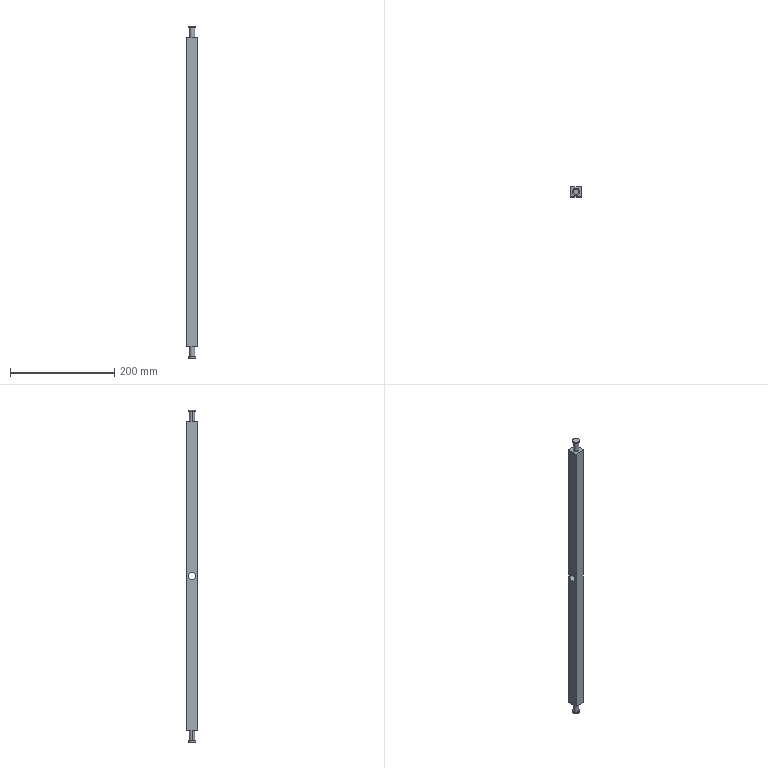Part | SolidWorks | 1 solid | 20 faces | box 20 x 20 x 638 mm | volume 238279 mm3 | cylinder 10 | plane 10 | commonest cylinder face diameters 14 x6 10 x4
STEP:
#1=CARTESIAN_POINT('',(-10.,-7.,0.));
#2=VERTEX_POINT('',#1);
#3=CARTESIAN_POINT('',(-10.,7.,0.));
#4=VERTEX_POINT('',#3);
#5=CARTESIAN_POINT('',(-10.,0.,0.));
#6=DIRECTION('',(1.,0.,0.));
#7=DIRECTION('',(0.,1.,0.));
#8=AXIS2_PLACEMENT_3D('',#5,#6,#7);
#9=CIRCLE('',#8,7.);
#10=EDGE_CURVE('',#2,#4,#9,.T.);
#11=ORIENTED_EDGE('',*,*,#10,.F.);
#12=CARTESIAN_POINT('',(10.,-7.,0.));
#13=VERTEX_POINT('',#12);
#14=CARTESIAN_POINT('',(-46.,-7.,0.));
#15=DIRECTION('',(1.,0.,0.));
#16=VECTOR('',#15,1000.);
#17=LINE('',#14,#16);
#18=EDGE_CURVE('',#2,#13,#17,.T.);
#19=ORIENTED_EDGE('',*,*,#18,.T.);
#20=CARTESIAN_POINT('',(10.,7.,0.));
#21=VERTEX_POINT('',#20);
#22=CARTESIAN_POINT('',(10.,0.,0.));
#23=DIRECTION('',(1.,0.,0.));
#24=DIRECTION('',(0.,1.,0.));
#25=AXIS2_PLACEMENT_3D('',#22,#23,#24);
#26=CIRCLE('',#25,7.);
#27=EDGE_CURVE('',#13,#21,#26,.T.);
#28=ORIENTED_EDGE('',*,*,#27,.T.);
#29=CARTESIAN_POINT('',(-46.,7.,0.));
#30=DIRECTION('',(1.,0.,0.));
#31=VECTOR('',#30,1000.);
#32=LINE('',#29,#31);
#33=EDGE_CURVE('',#4,#21,#32,.T.);
#34=ORIENTED_EDGE('',*,*,#33,.F.);
#35=EDGE_LOOP('',(#11,#19,#28,#34));
#36=FACE_OUTER_BOUND('',#35,.T.);
#37=CARTESIAN_POINT('',(-46.,0.,0.));
#38=DIRECTION('',(1.,0.,0.));
#39=DIRECTION('',(0.,1.,0.));
#40=AXIS2_PLACEMENT_3D('',#37,#38,#39);
#41=CYLINDRICAL_SURFACE('',#40,7.);
#42=ADVANCED_FACE('',(#36),#41,.F.);
#43=CARTESIAN_POINT('',(7.,0.,-319.));
#44=VERTEX_POINT('',#43);
#45=CARTESIAN_POINT('',(-7.,0.,-319.));
#46=VERTEX_POINT('',#45);
#47=CARTESIAN_POINT('',(0.,0.,-319.));
#48=DIRECTION('',(0.,0.,1.));
#49=DIRECTION('',(1.,0.,0.));
#50=AXIS2_PLACEMENT_3D('',#47,#48,#49);
#51=CIRCLE('',#50,7.);
#52=EDGE_CURVE('',#44,#46,#51,.T.);
#53=ORIENTED_EDGE('',*,*,#52,.T.);
#54=CARTESIAN_POINT('',(-7.,0.,-317.));
#55=VERTEX_POINT('',#54);
#56=CARTESIAN_POINT('',(-7.,0.,-319.));
#57=DIRECTION('',(0.,0.,1.));
#58=VECTOR('',#57,1000.);
#59=LINE('',#56,#58);
#60=EDGE_CURVE('',#46,#55,#59,.T.);
#61=ORIENTED_EDGE('',*,*,#60,.T.);
#62=CARTESIAN_POINT('',(7.,0.,-317.));
#63=VERTEX_POINT('',#62);
#64=CARTESIAN_POINT('',(0.,0.,-317.));
#65=DIRECTION('',(0.,0.,1.));
#66=DIRECTION('',(1.,0.,0.));
#67=AXIS2_PLACEMENT_3D('',#64,#65,#66);
#68=CIRCLE('',#67,7.);
#69=EDGE_CURVE('',#63,#55,#68,.T.);
#70=ORIENTED_EDGE('',*,*,#69,.F.);
#71=CARTESIAN_POINT('',(7.,0.,-319.));
#72=DIRECTION('',(0.,0.,1.));
#73=VECTOR('',#72,1000.);
#74=LINE('',#71,#73);
#75=EDGE_CURVE('',#44,#63,#74,.T.);
#76=ORIENTED_EDGE('',*,*,#75,.F.);
#77=EDGE_LOOP('',(#53,#61,#70,#76));
#78=FACE_OUTER_BOUND('',#77,.T.);
#79=CARTESIAN_POINT('',(0.,0.,-319.));
#80=DIRECTION('',(0.,0.,1.));
#81=DIRECTION('',(1.,0.,0.));
#82=AXIS2_PLACEMENT_3D('',#79,#80,#81);
#83=CYLINDRICAL_SURFACE('',#82,7.);
#84=ADVANCED_FACE('',(#78),#83,.T.);
#85=CARTESIAN_POINT('',(5.,0.,-317.));
#86=VERTEX_POINT('',#85);
#87=CARTESIAN_POINT('',(-5.,0.,-317.));
#88=VERTEX_POINT('',#87);
#89=CARTESIAN_POINT('',(0.,0.,-317.));
#90=DIRECTION('',(0.,0.,1.));
#91=DIRECTION('',(1.,0.,0.));
#92=AXIS2_PLACEMENT_3D('',#89,#90,#91);
#93=CIRCLE('',#92,5.);
#94=EDGE_CURVE('',#86,#88,#93,.T.);
#95=ORIENTED_EDGE('',*,*,#94,.T.);
#96=CARTESIAN_POINT('',(-5.,0.,-297.));
#97=VERTEX_POINT('',#96);
#98=CARTESIAN_POINT('',(-5.,0.,-317.));
#99=DIRECTION('',(0.,0.,1.));
#100=VECTOR('',#99,1000.);
#101=LINE('',#98,#100);
#102=EDGE_CURVE('',#88,#97,#101,.T.);
#103=ORIENTED_EDGE('',*,*,#102,.T.);
#104=CARTESIAN_POINT('',(5.,0.,-297.));
#105=VERTEX_POINT('',#104);
#106=CARTESIAN_POINT('',(0.,0.,-297.));
#107=DIRECTION('',(0.,0.,1.));
#108=DIRECTION('',(1.,0.,0.));
#109=AXIS2_PLACEMENT_3D('',#106,#107,#108);
#110=CIRCLE('',#109,5.);
#111=EDGE_CURVE('',#105,#97,#110,.T.);
#112=ORIENTED_EDGE('',*,*,#111,.F.);
#113=CARTESIAN_POINT('',(5.,0.,-317.));
#114=DIRECTION('',(0.,0.,1.));
#115=VECTOR('',#114,1000.);
#116=LINE('',#113,#115);
#117=EDGE_CURVE('',#86,#105,#116,.T.);
#118=ORIENTED_EDGE('',*,*,#117,.F.);
#119=EDGE_LOOP('',(#95,#103,#112,#118));
#120=FACE_OUTER_BOUND('',#119,.T.);
#121=CARTESIAN_POINT('',(0.,0.,-317.));
#122=DIRECTION('',(0.,0.,1.));
#123=DIRECTION('',(1.,0.,0.));
#124=AXIS2_PLACEMENT_3D('',#121,#122,#123);
#125=CYLINDRICAL_SURFACE('',#124,5.);
#126=ADVANCED_FACE('',(#120),#125,.T.);
#127=CARTESIAN_POINT('',(7.,0.,319.));
#128=VERTEX_POINT('',#127);
#129=CARTESIAN_POINT('',(-7.,0.,319.));
#130=VERTEX_POINT('',#129);
#131=CARTESIAN_POINT('',(0.,0.,319.));
#132=DIRECTION('',(0.,0.,1.));
#133=DIRECTION('',(1.,0.,0.));
#134=AXIS2_PLACEMENT_3D('',#131,#132,#133);
#135=CIRCLE('',#134,7.);
#136=EDGE_CURVE('',#128,#130,#135,.T.);
#137=ORIENTED_EDGE('',*,*,#136,.F.);
#138=CARTESIAN_POINT('',(7.,0.,317.));
#139=VERTEX_POINT('',#138);
#140=CARTESIAN_POINT('',(7.,0.,319.));
#141=DIRECTION('',(0.,0.,-1.));
#142=VECTOR('',#141,1000.);
#143=LINE('',#140,#142);
#144=EDGE_CURVE('',#128,#139,#143,.T.);
#145=ORIENTED_EDGE('',*,*,#144,.T.);
#146=CARTESIAN_POINT('',(-7.,0.,317.));
#147=VERTEX_POINT('',#146);
#148=CARTESIAN_POINT('',(0.,0.,317.));
#149=DIRECTION('',(0.,0.,1.));
#150=DIRECTION('',(1.,0.,0.));
#151=AXIS2_PLACEMENT_3D('',#148,#149,#150);
#152=CIRCLE('',#151,7.);
#153=EDGE_CURVE('',#139,#147,#152,.T.);
#154=ORIENTED_EDGE('',*,*,#153,.T.);
#155=CARTESIAN_POINT('',(-7.,0.,319.));
#156=DIRECTION('',(0.,0.,-1.));
#157=VECTOR('',#156,1000.);
#158=LINE('',#155,#157);
#159=EDGE_CURVE('',#130,#147,#158,.T.);
#160=ORIENTED_EDGE('',*,*,#159,.F.);
#161=EDGE_LOOP('',(#137,#145,#154,#160));
#162=FACE_OUTER_BOUND('',#161,.T.);
#163=CARTESIAN_POINT('',(0.,0.,319.));
#164=DIRECTION('',(0.,0.,-1.));
#165=DIRECTION('',(-1.,0.,0.));
#166=AXIS2_PLACEMENT_3D('',#163,#164,#165);
#167=CYLINDRICAL_SURFACE('',#166,7.);
#168=ADVANCED_FACE('',(#162),#167,.T.);
#169=CARTESIAN_POINT('',(5.,0.,317.));
#170=VERTEX_POINT('',#169);
#171=CARTESIAN_POINT('',(-5.,0.,317.));
#172=VERTEX_POINT('',#171);
#173=CARTESIAN_POINT('',(0.,0.,317.));
#174=DIRECTION('',(0.,0.,1.));
#175=DIRECTION('',(1.,0.,0.));
#176=AXIS2_PLACEMENT_3D('',#173,#174,#175);
#177=CIRCLE('',#176,5.);
#178=EDGE_CURVE('',#170,#172,#177,.T.);
#179=ORIENTED_EDGE('',*,*,#178,.F.);
#180=CARTESIAN_POINT('',(5.,0.,297.));
#181=VERTEX_POINT('',#180);
#182=CARTESIAN_POINT('',(5.,0.,317.));
#183=DIRECTION('',(0.,0.,-1.));
#184=VECTOR('',#183,1000.);
#185=LINE('',#182,#184);
#186=EDGE_CURVE('',#170,#181,#185,.T.);
#187=ORIENTED_EDGE('',*,*,#186,.T.);
#188=CARTESIAN_POINT('',(-5.,0.,297.));
#189=VERTEX_POINT('',#188);
#190=CARTESIAN_POINT('',(0.,0.,297.));
#191=DIRECTION('',(0.,0.,1.));
#192=DIRECTION('',(1.,0.,0.));
#193=AXIS2_PLACEMENT_3D('',#190,#191,#192);
#194=CIRCLE('',#193,5.);
#195=EDGE_CURVE('',#181,#189,#194,.T.);
#196=ORIENTED_EDGE('',*,*,#195,.T.);
#197=CARTESIAN_POINT('',(-5.,0.,317.));
#198=DIRECTION('',(0.,0.,-1.));
#199=VECTOR('',#198,1000.);
#200=LINE('',#197,#199);
#201=EDGE_CURVE('',#172,#189,#200,.T.);
#202=ORIENTED_EDGE('',*,*,#201,.F.);
#203=EDGE_LOOP('',(#179,#187,#196,#202));
#204=FACE_OUTER_BOUND('',#203,.T.);
#205=CARTESIAN_POINT('',(0.,0.,317.));
#206=DIRECTION('',(0.,0.,-1.));
#207=DIRECTION('',(-1.,0.,0.));
#208=AXIS2_PLACEMENT_3D('',#205,#206,#207);
#209=CYLINDRICAL_SURFACE('',#208,5.);
#210=ADVANCED_FACE('',(#204),#209,.T.);
#211=CARTESIAN_POINT('',(10.,0.,0.));
#212=DIRECTION('',(1.,0.,0.));
#213=DIRECTION('',(0.,1.,0.));
#214=AXIS2_PLACEMENT_3D('',#211,#212,#213);
#215=CIRCLE('',#214,7.);
#216=EDGE_CURVE('',#21,#13,#215,.T.);
#217=ORIENTED_EDGE('',*,*,#216,.F.);
#218=ORIENTED_EDGE('',*,*,#27,.F.);
#219=EDGE_LOOP('',(#217,#218));
#220=FACE_BOUND('',#219,.T.);
#221=CARTESIAN_POINT('',(10.,-10.,-297.));
#222=VERTEX_POINT('',#221);
#223=CARTESIAN_POINT('',(10.,10.,-297.));
#224=VERTEX_POINT('',#223);
#225=CARTESIAN_POINT('',(10.,10.,-297.));
#226=DIRECTION('',(0.,1.,0.));
#227=VECTOR('',#226,1000.);
#228=LINE('',#225,#227);
#229=EDGE_CURVE('',#222,#224,#228,.T.);
#230=ORIENTED_EDGE('',*,*,#229,.T.);
#231=CARTESIAN_POINT('',(10.,10.,297.));
#232=VERTEX_POINT('',#231);
#233=CARTESIAN_POINT('',(10.,10.,297.));
#234=DIRECTION('',(0.,0.,-1.));
#235=VECTOR('',#234,1000.);
#236=LINE('',#233,#235);
#237=EDGE_CURVE('',#232,#224,#236,.T.);
#238=ORIENTED_EDGE('',*,*,#237,.F.);
#239=CARTESIAN_POINT('',(10.,-10.,297.));
#240=VERTEX_POINT('',#239);
#241=CARTESIAN_POINT('',(10.,10.,297.));
#242=DIRECTION('',(0.,1.,0.));
#243=VECTOR('',#242,1000.);
#244=LINE('',#241,#243);
#245=EDGE_CURVE('',#240,#232,#244,.T.);
#246=ORIENTED_EDGE('',*,*,#245,.F.);
#247=CARTESIAN_POINT('',(10.,-10.,297.));
#248=DIRECTION('',(0.,0.,-1.));
#249=VECTOR('',#248,1000.);
#250=LINE('',#247,#249);
#251=EDGE_CURVE('',#240,#222,#250,.T.);
#252=ORIENTED_EDGE('',*,*,#251,.T.);
#253=EDGE_LOOP('',(#230,#238,#246,#252));
#254=FACE_OUTER_BOUND('',#253,.T.);
#255=CARTESIAN_POINT('',(10.,10.,297.));
#256=DIRECTION('',(-1.,0.,0.));
#257=DIRECTION('',(0.,-1.,0.));
#258=AXIS2_PLACEMENT_3D('',#255,#256,#257);
#259=PLANE('',#258);
#260=ADVANCED_FACE('',(#220,#254),#259,.F.);
#261=CARTESIAN_POINT('',(-10.,10.,-297.));
#262=VERTEX_POINT('',#261);
#263=CARTESIAN_POINT('',(-10.,10.,-297.));
#264=DIRECTION('',(-1.,0.,0.));
#265=VECTOR('',#264,1000.);
#266=LINE('',#263,#265);
#267=EDGE_CURVE('',#224,#262,#266,.T.);
#268=ORIENTED_EDGE('',*,*,#267,.T.);
#269=CARTESIAN_POINT('',(-10.,10.,297.));
#270=VERTEX_POINT('',#269);
#271=CARTESIAN_POINT('',(-10.,10.,297.));
#272=DIRECTION('',(0.,0.,-1.));
#273=VECTOR('',#272,1000.);
#274=LINE('',#271,#273);
#275=EDGE_CURVE('',#270,#262,#274,.T.);
#276=ORIENTED_EDGE('',*,*,#275,.F.);
#277=CARTESIAN_POINT('',(-10.,10.,297.));
#278=DIRECTION('',(-1.,0.,0.));
#279=VECTOR('',#278,1000.);
#280=LINE('',#277,#279);
#281=EDGE_CURVE('',#232,#270,#280,.T.);
#282=ORIENTED_EDGE('',*,*,#281,.F.);
#283=ORIENTED_EDGE('',*,*,#237,.T.);
#284=EDGE_LOOP('',(#268,#276,#282,#283));
#285=FACE_OUTER_BOUND('',#284,.T.);
#286=CARTESIAN_POINT('',(-10.,10.,297.));
#287=DIRECTION('',(0.,-1.,0.));
#288=DIRECTION('',(0.,0.,-1.));
#289=AXIS2_PLACEMENT_3D('',#286,#287,#288);
#290=PLANE('',#289);
#291=ADVANCED_FACE('',(#285),#290,.F.);
#292=CARTESIAN_POINT('',(-10.,0.,0.));
#293=DIRECTION('',(1.,0.,0.));
#294=DIRECTION('',(0.,1.,0.));
#295=AXIS2_PLACEMENT_3D('',#292,#293,#294);
#296=CIRCLE('',#295,7.);
#297=EDGE_CURVE('',#4,#2,#296,.T.);
#298=ORIENTED_EDGE('',*,*,#297,.T.);
#299=ORIENTED_EDGE('',*,*,#10,.T.);
#300=EDGE_LOOP('',(#298,#299));
#301=FACE_BOUND('',#300,.T.);
#302=CARTESIAN_POINT('',(-10.,-10.,-297.));
#303=VERTEX_POINT('',#302);
#304=CARTESIAN_POINT('',(-10.,10.,-297.));
#305=DIRECTION('',(0.,-1.,0.));
#306=VECTOR('',#305,1000.);
#307=LINE('',#304,#306);
#308=EDGE_CURVE('',#262,#303,#307,.T.);
#309=ORIENTED_EDGE('',*,*,#308,.T.);
#310=CARTESIAN_POINT('',(-10.,-10.,297.));
#311=VERTEX_POINT('',#310);
#312=CARTESIAN_POINT('',(-10.,-10.,297.));
#313=DIRECTION('',(0.,0.,-1.));
#314=VECTOR('',#313,1000.);
#315=LINE('',#312,#314);
#316=EDGE_CURVE('',#311,#303,#315,.T.);
#317=ORIENTED_EDGE('',*,*,#316,.F.);
#318=CARTESIAN_POINT('',(-10.,10.,297.));
#319=DIRECTION('',(0.,-1.,0.));
#320=VECTOR('',#319,1000.);
#321=LINE('',#318,#320);
#322=EDGE_CURVE('',#270,#311,#321,.T.);
#323=ORIENTED_EDGE('',*,*,#322,.F.);
#324=ORIENTED_EDGE('',*,*,#275,.T.);
#325=EDGE_LOOP('',(#309,#317,#323,#324));
#326=FACE_OUTER_BOUND('',#325,.T.);
#327=CARTESIAN_POINT('',(-10.,10.,297.));
#328=DIRECTION('',(1.,0.,0.));
#329=DIRECTION('',(0.,1.,0.));
#330=AXIS2_PLACEMENT_3D('',#327,#328,#329);
#331=PLANE('',#330);
#332=ADVANCED_FACE('',(#301,#326),#331,.F.);
#333=CARTESIAN_POINT('',(-10.,-10.,-297.));
#334=DIRECTION('',(1.,0.,0.));
#335=VECTOR('',#334,1000.);
#336=LINE('',#333,#335);
#337=EDGE_CURVE('',#303,#222,#336,.T.);
#338=ORIENTED_EDGE('',*,*,#337,.T.);
#339=ORIENTED_EDGE('',*,*,#251,.F.);
#340=CARTESIAN_POINT('',(-10.,-10.,297.));
#341=DIRECTION('',(1.,0.,0.));
#342=VECTOR('',#341,1000.);
#343=LINE('',#340,#342);
#344=EDGE_CURVE('',#311,#240,#343,.T.);
#345=ORIENTED_EDGE('',*,*,#344,.F.);
#346=ORIENTED_EDGE('',*,*,#316,.T.);
#347=EDGE_LOOP('',(#338,#339,#345,#346));
#348=FACE_OUTER_BOUND('',#347,.T.);
#349=CARTESIAN_POINT('',(-10.,-10.,297.));
#350=DIRECTION('',(0.,1.,0.));
#351=DIRECTION('',(0.,0.,1.));
#352=AXIS2_PLACEMENT_3D('',#349,#350,#351);
#353=PLANE('',#352);
#354=ADVANCED_FACE('',(#348),#353,.F.);
#355=CARTESIAN_POINT('',(0.,0.,297.));
#356=DIRECTION('',(0.,0.,1.));
#357=DIRECTION('',(1.,0.,0.));
#358=AXIS2_PLACEMENT_3D('',#355,#356,#357);
#359=CIRCLE('',#358,5.);
#360=EDGE_CURVE('',#189,#181,#359,.T.);
#361=ORIENTED_EDGE('',*,*,#360,.F.);
#362=ORIENTED_EDGE('',*,*,#195,.F.);
#363=EDGE_LOOP('',(#361,#362));
#364=FACE_BOUND('',#363,.T.);
#365=ORIENTED_EDGE('',*,*,#245,.T.);
#366=ORIENTED_EDGE('',*,*,#281,.T.);
#367=ORIENTED_EDGE('',*,*,#322,.T.);
#368=ORIENTED_EDGE('',*,*,#344,.T.);
#369=EDGE_LOOP('',(#365,#366,#367,#368));
#370=FACE_OUTER_BOUND('',#369,.T.);
#371=CARTESIAN_POINT('',(0.,0.,297.));
#372=DIRECTION('',(0.,0.,1.));
#373=DIRECTION('',(1.,0.,0.));
#374=AXIS2_PLACEMENT_3D('',#371,#372,#373);
#375=PLANE('',#374);
#376=ADVANCED_FACE('',(#364,#370),#375,.T.);
#377=ORIENTED_EDGE('',*,*,#111,.T.);
#378=CARTESIAN_POINT('',(0.,0.,-297.));
#379=DIRECTION('',(0.,0.,1.));
#380=DIRECTION('',(1.,0.,0.));
#381=AXIS2_PLACEMENT_3D('',#378,#379,#380);
#382=CIRCLE('',#381,5.);
#383=EDGE_CURVE('',#97,#105,#382,.T.);
#384=ORIENTED_EDGE('',*,*,#383,.T.);
#385=EDGE_LOOP('',(#377,#384));
#386=FACE_BOUND('',#385,.T.);
#387=ORIENTED_EDGE('',*,*,#229,.F.);
#388=ORIENTED_EDGE('',*,*,#337,.F.);
#389=ORIENTED_EDGE('',*,*,#308,.F.);
#390=ORIENTED_EDGE('',*,*,#267,.F.);
#391=EDGE_LOOP('',(#387,#388,#389,#390));
#392=FACE_OUTER_BOUND('',#391,.T.);
#393=CARTESIAN_POINT('',(0.,0.,-297.));
#394=DIRECTION('',(0.,0.,1.));
#395=DIRECTION('',(1.,0.,0.));
#396=AXIS2_PLACEMENT_3D('',#393,#394,#395);
#397=PLANE('',#396);
#398=ADVANCED_FACE('',(#386,#392),#397,.F.);
#399=ORIENTED_EDGE('',*,*,#186,.F.);
#400=CARTESIAN_POINT('',(0.,0.,317.));
#401=DIRECTION('',(0.,0.,1.));
#402=DIRECTION('',(1.,0.,0.));
#403=AXIS2_PLACEMENT_3D('',#400,#401,#402);
#404=CIRCLE('',#403,5.);
#405=EDGE_CURVE('',#172,#170,#404,.T.);
#406=ORIENTED_EDGE('',*,*,#405,.F.);
#407=ORIENTED_EDGE('',*,*,#201,.T.);
#408=ORIENTED_EDGE('',*,*,#360,.T.);
#409=EDGE_LOOP('',(#399,#406,#407,#408));
#410=FACE_OUTER_BOUND('',#409,.T.);
#411=CARTESIAN_POINT('',(0.,0.,317.));
#412=DIRECTION('',(0.,0.,-1.));
#413=DIRECTION('',(-1.,0.,0.));
#414=AXIS2_PLACEMENT_3D('',#411,#412,#413);
#415=CYLINDRICAL_SURFACE('',#414,5.);
#416=ADVANCED_FACE('',(#410),#415,.T.);
#417=ORIENTED_EDGE('',*,*,#144,.F.);
#418=CARTESIAN_POINT('',(0.,0.,319.));
#419=DIRECTION('',(0.,0.,1.));
#420=DIRECTION('',(1.,0.,0.));
#421=AXIS2_PLACEMENT_3D('',#418,#419,#420);
#422=CIRCLE('',#421,7.);
#423=EDGE_CURVE('',#130,#128,#422,.T.);
#424=ORIENTED_EDGE('',*,*,#423,.F.);
#425=ORIENTED_EDGE('',*,*,#159,.T.);
#426=CARTESIAN_POINT('',(0.,0.,317.));
#427=DIRECTION('',(0.,0.,1.));
#428=DIRECTION('',(1.,0.,0.));
#429=AXIS2_PLACEMENT_3D('',#426,#427,#428);
#430=CIRCLE('',#429,7.);
#431=EDGE_CURVE('',#147,#139,#430,.T.);
#432=ORIENTED_EDGE('',*,*,#431,.T.);
#433=EDGE_LOOP('',(#417,#424,#425,#432));
#434=FACE_OUTER_BOUND('',#433,.T.);
#435=CARTESIAN_POINT('',(0.,0.,319.));
#436=DIRECTION('',(0.,0.,-1.));
#437=DIRECTION('',(-1.,0.,0.));
#438=AXIS2_PLACEMENT_3D('',#435,#436,#437);
#439=CYLINDRICAL_SURFACE('',#438,7.);
#440=ADVANCED_FACE('',(#434),#439,.T.);
#441=ORIENTED_EDGE('',*,*,#423,.T.);
#442=ORIENTED_EDGE('',*,*,#136,.T.);
#443=EDGE_LOOP('',(#441,#442));
#444=FACE_OUTER_BOUND('',#443,.T.);
#445=CARTESIAN_POINT('',(0.,0.,319.));
#446=DIRECTION('',(0.,0.,1.));
#447=DIRECTION('',(1.,0.,0.));
#448=AXIS2_PLACEMENT_3D('',#445,#446,#447);
#449=PLANE('',#448);
#450=ADVANCED_FACE('',(#444),#449,.T.);
#451=ORIENTED_EDGE('',*,*,#405,.T.);
#452=ORIENTED_EDGE('',*,*,#178,.T.);
#453=EDGE_LOOP('',(#451,#452));
#454=FACE_BOUND('',#453,.T.);
#455=ORIENTED_EDGE('',*,*,#431,.F.);
#456=ORIENTED_EDGE('',*,*,#153,.F.);
#457=EDGE_LOOP('',(#455,#456));
#458=FACE_OUTER_BOUND('',#457,.T.);
#459=CARTESIAN_POINT('',(0.,0.,317.));
#460=DIRECTION('',(0.,0.,1.));
#461=DIRECTION('',(1.,0.,0.));
#462=AXIS2_PLACEMENT_3D('',#459,#460,#461);
#463=PLANE('',#462);
#464=ADVANCED_FACE('',(#454,#458),#463,.F.);
#465=ORIENTED_EDGE('',*,*,#102,.F.);
#466=CARTESIAN_POINT('',(0.,0.,-317.));
#467=DIRECTION('',(0.,0.,1.));
#468=DIRECTION('',(1.,0.,0.));
#469=AXIS2_PLACEMENT_3D('',#466,#467,#468);
#470=CIRCLE('',#469,5.);
#471=EDGE_CURVE('',#88,#86,#470,.T.);
#472=ORIENTED_EDGE('',*,*,#471,.T.);
#473=ORIENTED_EDGE('',*,*,#117,.T.);
#474=ORIENTED_EDGE('',*,*,#383,.F.);
#475=EDGE_LOOP('',(#465,#472,#473,#474));
#476=FACE_OUTER_BOUND('',#475,.T.);
#477=CARTESIAN_POINT('',(0.,0.,-317.));
#478=DIRECTION('',(0.,0.,1.));
#479=DIRECTION('',(1.,0.,0.));
#480=AXIS2_PLACEMENT_3D('',#477,#478,#479);
#481=CYLINDRICAL_SURFACE('',#480,5.);
#482=ADVANCED_FACE('',(#476),#481,.T.);
#483=ORIENTED_EDGE('',*,*,#60,.F.);
#484=CARTESIAN_POINT('',(0.,0.,-319.));
#485=DIRECTION('',(0.,0.,1.));
#486=DIRECTION('',(1.,0.,0.));
#487=AXIS2_PLACEMENT_3D('',#484,#485,#486);
#488=CIRCLE('',#487,7.);
#489=EDGE_CURVE('',#46,#44,#488,.T.);
#490=ORIENTED_EDGE('',*,*,#489,.T.);
#491=ORIENTED_EDGE('',*,*,#75,.T.);
#492=CARTESIAN_POINT('',(0.,0.,-317.));
#493=DIRECTION('',(0.,0.,1.));
#494=DIRECTION('',(1.,0.,0.));
#495=AXIS2_PLACEMENT_3D('',#492,#493,#494);
#496=CIRCLE('',#495,7.);
#497=EDGE_CURVE('',#55,#63,#496,.T.);
#498=ORIENTED_EDGE('',*,*,#497,.F.);
#499=EDGE_LOOP('',(#483,#490,#491,#498));
#500=FACE_OUTER_BOUND('',#499,.T.);
#501=CARTESIAN_POINT('',(0.,0.,-319.));
#502=DIRECTION('',(0.,0.,1.));
#503=DIRECTION('',(1.,0.,0.));
#504=AXIS2_PLACEMENT_3D('',#501,#502,#503);
#505=CYLINDRICAL_SURFACE('',#504,7.);
#506=ADVANCED_FACE('',(#500),#505,.T.);
#507=ORIENTED_EDGE('',*,*,#52,.F.);
#508=ORIENTED_EDGE('',*,*,#489,.F.);
#509=EDGE_LOOP('',(#507,#508));
#510=FACE_OUTER_BOUND('',#509,.T.);
#511=CARTESIAN_POINT('',(0.,0.,-319.));
#512=DIRECTION('',(0.,0.,-1.));
#513=DIRECTION('',(1.,0.,0.));
#514=AXIS2_PLACEMENT_3D('',#511,#512,#513);
#515=PLANE('',#514);
#516=ADVANCED_FACE('',(#510),#515,.T.);
#517=ORIENTED_EDGE('',*,*,#94,.F.);
#518=ORIENTED_EDGE('',*,*,#471,.F.);
#519=EDGE_LOOP('',(#517,#518));
#520=FACE_BOUND('',#519,.T.);
#521=ORIENTED_EDGE('',*,*,#69,.T.);
#522=ORIENTED_EDGE('',*,*,#497,.T.);
#523=EDGE_LOOP('',(#521,#522));
#524=FACE_OUTER_BOUND('',#523,.T.);
#525=CARTESIAN_POINT('',(0.,0.,-317.));
#526=DIRECTION('',(0.,0.,-1.));
#527=DIRECTION('',(1.,0.,0.));
#528=AXIS2_PLACEMENT_3D('',#525,#526,#527);
#529=PLANE('',#528);
#530=ADVANCED_FACE('',(#520,#524),#529,.F.);
#531=ORIENTED_EDGE('',*,*,#18,.F.);
#532=ORIENTED_EDGE('',*,*,#297,.F.);
#533=ORIENTED_EDGE('',*,*,#33,.T.);
#534=ORIENTED_EDGE('',*,*,#216,.T.);
#535=EDGE_LOOP('',(#531,#532,#533,#534));
#536=FACE_OUTER_BOUND('',#535,.T.);
#537=CARTESIAN_POINT('',(-46.,0.,0.));
#538=DIRECTION('',(1.,0.,0.));
#539=DIRECTION('',(0.,1.,0.));
#540=AXIS2_PLACEMENT_3D('',#537,#538,#539);
#541=CYLINDRICAL_SURFACE('',#540,7.);
#542=ADVANCED_FACE('',(#536),#541,.F.);
#543=CLOSED_SHELL('',(#42,#84,#126,#168,#210,#260,#291,#332,#354,#376,#398,#416,#440,#450,#464,#482,#506,#516,#530,#542));
#544=MANIFOLD_SOLID_BREP('',#543);
#545=CARTESIAN_POINT('',(0.,0.,0.));
#546=DIRECTION('',(0.,0.,1.));
#547=DIRECTION('',(1.,0.,0.));
#548=AXIS2_PLACEMENT_3D('',#545,#546,#547);
#549=(LENGTH_UNIT()NAMED_UNIT(*)SI_UNIT(.MILLI.,.METRE.));
#550=UNCERTAINTY_MEASURE_WITH_UNIT(LENGTH_MEASURE(0.00001),#549,'','');
#551=(NAMED_UNIT(*)PLANE_ANGLE_UNIT()SI_UNIT($,.RADIAN.));
#552=(NAMED_UNIT(*)SI_UNIT($,.STERADIAN.)SOLID_ANGLE_UNIT());
#553=(GEOMETRIC_REPRESENTATION_CONTEXT(3)GLOBAL_UNCERTAINTY_ASSIGNED_CONTEXT((#550))GLOBAL_UNIT_ASSIGNED_CONTEXT((#549,#551,#552))REPRESENTATION_CONTEXT('',''));
#554=ADVANCED_BREP_SHAPE_REPRESENTATION('',(#544,#548),#553);